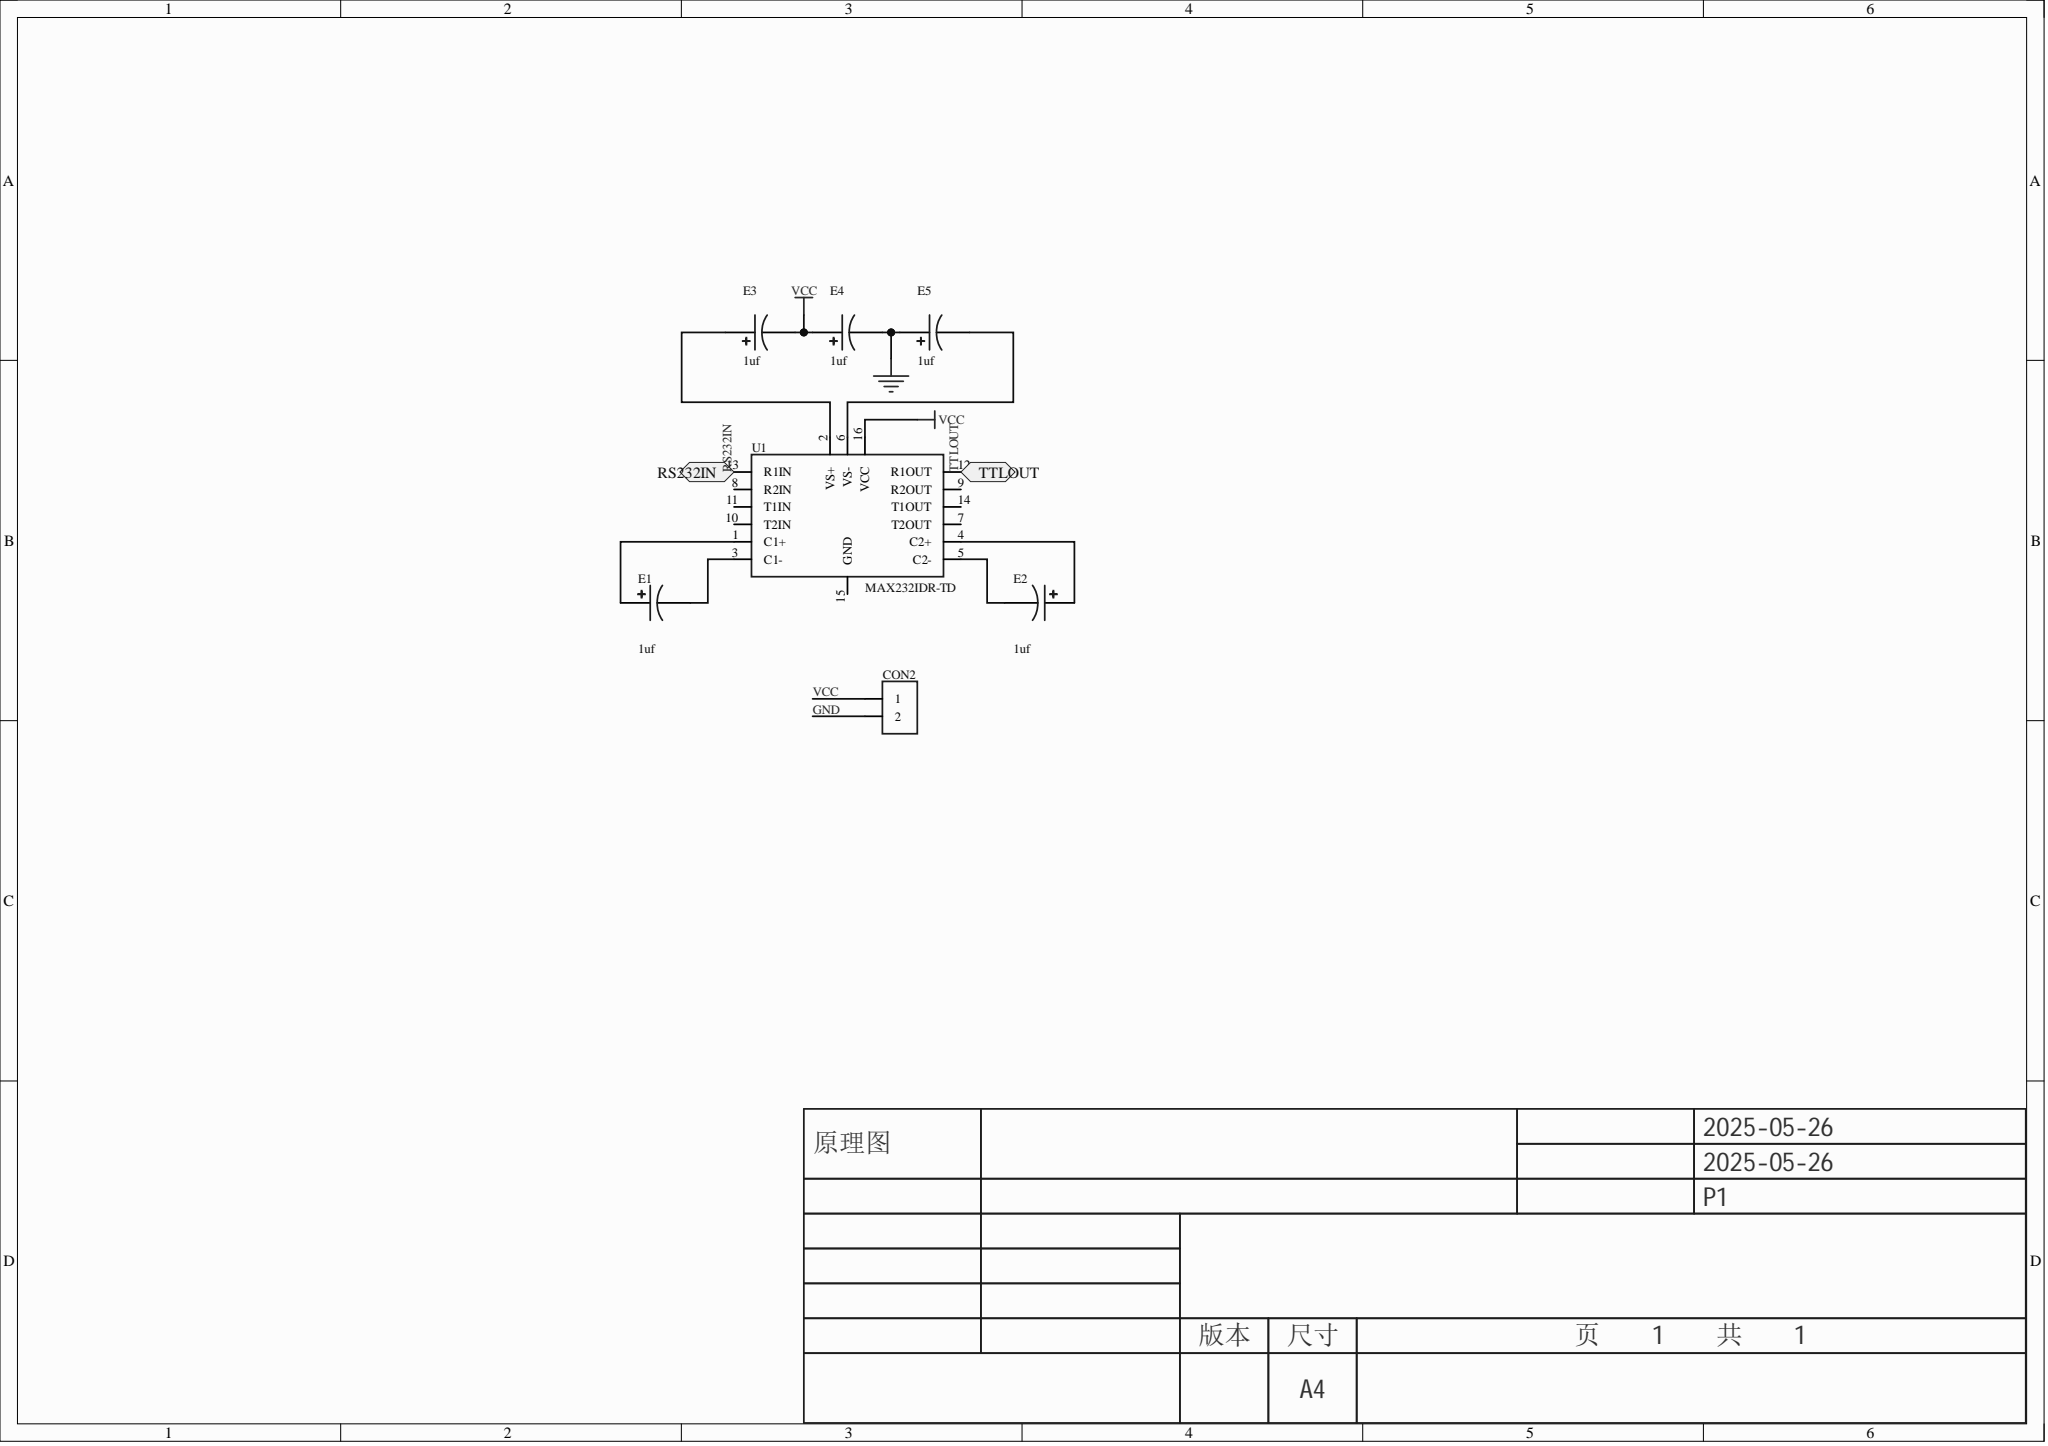Circuit board | Altium Designer | 7 parts | 8 nets
Bill of materials:
Comment,Description,Designator,Footprint,LibRef,Quantity
"","","CON2","SIP-2_L2.0-W1.1-P0.90-D0.3","HDR-F_2.54_1x2P","1"
"1uf","","E1, E2, E3, E4, E5","CAP-TH_L17.0-W10.4-P5.08_CDK11A_470UF","10uf","5"
"MAX232IDR-TD","类型:收发器;数据速率:120Kbps;","U1","DIP-16_L19.7-W6.6-P2.54-LS10.9-BL","MAX232IDR-TD","1"
Netlist (Protel format):
[
CON2
SIP-2_L2.0-W1.1-P0.90-D0.3




]
[
E1
CAP-TH_L17.0-W10.4-P5.08_CDK11A_470UF
1uf



]
[
E2
CAP-TH_L17.0-W10.4-P5.08_CDK11A_470UF
1uf



]
[
E3
CAP-TH_L17.0-W10.4-P5.08_CDK11A_470UF
1uf



]
[
E4
CAP-TH_L17.0-W10.4-P5.08_CDK11A_470UF
1uf



]
[
E5
CAP-TH_L17.0-W10.4-P5.08_CDK11A_470UF
1uf



]
[
U1
DIP-16_L19.7-W6.6-P2.54-LS10.9-BL
MAX232IDR-TD



]
(
VCC
CON2-1
E3-2
E4-1
U1-16
)
(
NetE5_2
E5-2
U1-6
)
(
NetE3_1
E3-1
U1-2
)
(
NetE2_2
E2-2
U1-5
)
(
NetE2_1
E2-1
U1-4
)
(
NetE1_2
E1-2
U1-3
)
(
NetE1_1
E1-1
U1-1
)
(
GND
CON2-2
E4-2
E5-1
)